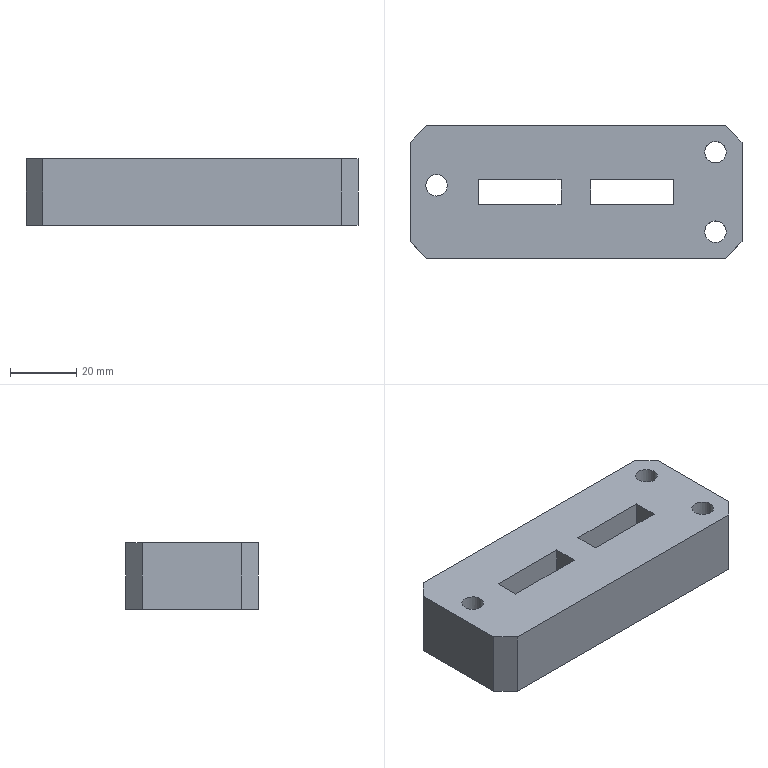Part | STEP file | P011002L005-001 | 1 solid | 27 faces | box 100 x 40 x 20 mm | volume 68887 mm3 | plane 11 | spline 10 | cylinder 6 | commonest cylinder face diameters 6.5 x3 9.5 x3